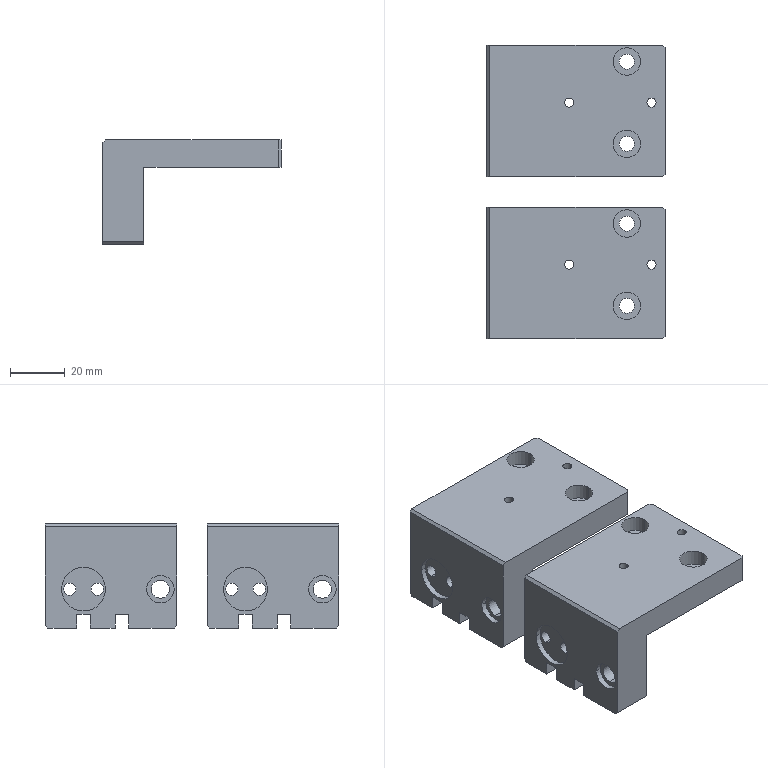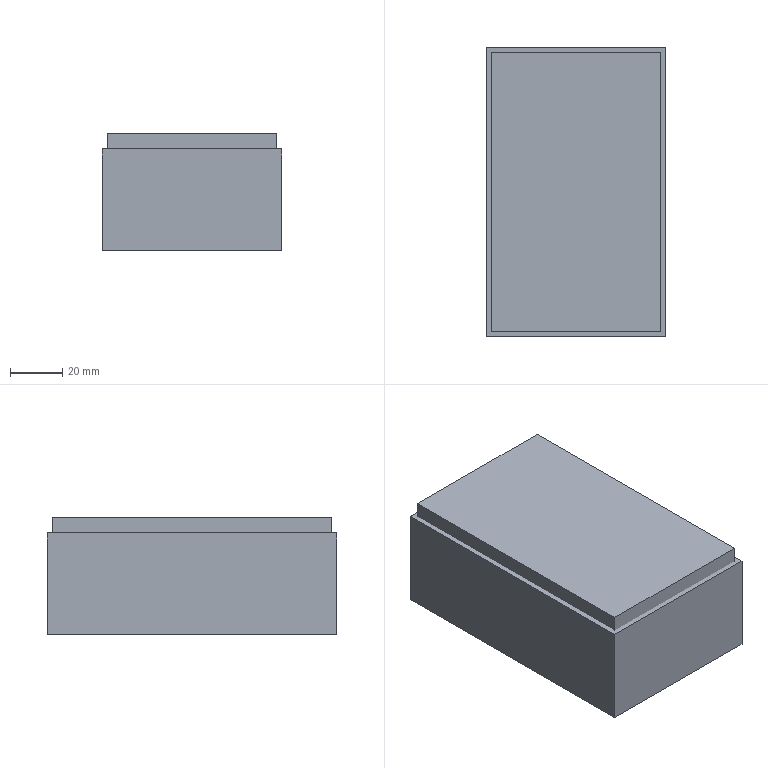CAM job | NX | 3+2 milling, drilling | part box 65 x 107 x 38 mm | stock box 69 x 111 x 45 mm
Tools:
number,name,description,diameter,corner_radius,flute_length,length,flutes
19,D80,Milling Tool-5 Parameters,80.0,0.0,50.0,75.0,2
1,D6A45,Milling Tool-5 Parameters,6.0,0.0,50.0,75.0,2
3,3.3ZT,Drilling Tool,3.3,0.0,35.0,50.0,2
8,4.5ZT,Drilling Tool,4.5,0.0,35.0,50.0,2
9,5.5ZT,Drilling Tool,5.5,0.0,35.0,50.0,2
15,D10,Milling Tool-5 Parameters,10.0,0.0,50.0,75.0,2
14,D10JING,Milling Tool-5 Parameters,10.0,0.0,50.0,75.0,2
12,D6,Milling Tool-5 Parameters,6.0,0.0,50.0,75.0,2
11,D4,Milling Tool-5 Parameters,4.0,0.0,50.0,75.0,2
10,6.6ZT,Drilling Tool,6.6,0.0,35.0,50.0,2
Operations:
program,operation,operation_type,tool,method,geometry_group,spindle_rpm,surface_speed,feed_per_tooth,feed_cut,feed_plunge,cut_length_mm,path_length_mm,cut_time_min,machine_time_min
1,FLOOR_WALL,VolumeBased25DMillingOperation,D80,METHOD,A,6500.0,1633.0,0.1154,1500.0,100.0,203.0,257.0,0.1353,0.1407
1,DRILLING,Operation,D6A45,METHOD,A,5000.0,94.0,0.035,350.0,0.0,32.0,297.109,0.0914,0.1179
1,DRILLING_COPY_1,Operation,3.3ZT,METHOD,A,2000.0,20.0,0.05,200.0,0.0,61.966,312.307,0.3098,0.3349
1,DRILLING_COPY_COPY_COPY,Operation,5.5ZT,METHOD,A,2000.0,26.0,0.075,300.0,0.0,62.609,283.673,0.2087,0.2308
1,ZLEVEL_PROFILE,ZLevelMilling,D10,METHOD,A,9500.0,298.0,0.1579,3000.0,1000.0,20133.797,20481.351,6.775,6.81
1,ZLEVEL_PROFILE_COPY_1,ZLevelMilling,D10JING,METHOD,A,9500.0,298.0,0.0632,1200.0,1000.0,2325.248,2620.577,2.068,2.098
1,HOLE_MILLING,CylinderMilling,D6,METHOD,A,9500.0,179.0,0.0789,1500.0,100.0,699.183,1048.983,0.4661,0.5011
1,PLANAR_MILL_COPY_COPY_COPY,PlanarMilling,D6A45,METHOD,A,9500.0,179.0,0.0658,1250.0,100.0,629.615,1415.04,0.5037,0.5822
1,PLANAR_MILL_COPY_COPY_COPY_COPY_1,PlanarMilling,D6A45,METHOD,A,9500.0,179.0,0.0658,1250.0,100.0,106.189,235.457,0.085,0.0979
1,PLANAR_MILL_COPY_COPY_COPY_COPY_1_COPY,PlanarMilling,D6A45,METHOD,A,9500.0,179.0,0.0658,1250.0,100.0,37.552,397.053,0.03,0.066
2,FLOOR_WALL_COPY,VolumeBased25DMillingOperation,D80,METHOD,B,6500.0,1633.0,0.1154,1500.0,100.0,1393.0,2887.002,0.9287,1.078
2,FLOOR_WALL_1,VolumeBased25DMillingOperation,D10,METHOD,B,9500.0,298.0,0.1842,3500.0,1000.0,23342.049,23881.836,6.687,6.741
2,FLOOR_WALL_2,VolumeBased25DMillingOperation,D10JING,METHOD,B,9500.0,298.0,0.0789,1500.0,100.0,1429.476,2061.769,0.953,1.016
2,FLOOR_WALL_2_COPY,VolumeBased25DMillingOperation,D10JING,METHOD,B,9500.0,298.0,0.0789,1500.0,100.0,247.472,828.328,0.165,0.2231
2,FLOOR_WALL_3,VolumeBased25DMillingOperation,D4,METHOD,B,9500.0,119.0,0.0789,1500.0,100.0,2496.0,2825.0,1.664,1.697
2,PLANAR_MILL_COPY_COPY_COPY_COPY,PlanarMilling,D6A45,METHOD,B,9500.0,179.0,0.0658,1250.0,100.0,396.496,855.836,0.3172,0.3631
2,PLANAR_MILL_COPY_COPY_COPY_COPY_COPY,PlanarMilling,D6A45,METHOD,B,9500.0,179.0,0.0658,1250.0,100.0,484.119,2362.262,0.3873,0.5751
3,DRILLING_COPY,Operation,D6A45,METHOD,C,5000.0,94.0,0.035,350.0,0.0,12.0,123.635,0.0343,0.0454
3,DRILLING_COPY_COPY_COPY_1,Operation,4.5ZT,METHOD,C,2000.0,26.0,0.075,300.0,0.0,40.704,154.848,0.1357,0.1471
3,DRILLING_COPY_COPY_COPY_1_COPY,Operation,6.6ZT,METHOD,C,2000.0,26.0,0.075,300.0,0.0,20.983,101.966,0.0699,0.078
3,HOLE_MILLING_COPY,CylinderMilling,D6,METHOD,C,9500.0,179.0,0.0789,1500.0,100.0,377.89,531.39,0.2519,0.2673
3,PLANAR_MILL_COPY_COPY_COPY_COPY_COPY_1,PlanarMilling,D6A45,METHOD,C,9500.0,179.0,0.0658,1250.0,100.0,85.152,232.566,0.0681,0.0829
3,刀补,CylinderMilling,D6,METHOD,C,9500.0,179.0,0.0789,1500.0,100.0,118.521,269.521,0.079,0.0941
4,HOLE_MILLING_COPY_1,CylinderMilling,D6,METHOD,D,9500.0,179.0,0.0263,500.0,100.0,253.014,419.314,0.506,0.5227
4,HOLE_MILLING_COPY_1_COPY,CylinderMilling,D6,METHOD,D,9500.0,179.0,0.0263,500.0,100.0,147.432,485.632,0.2949,0.3287